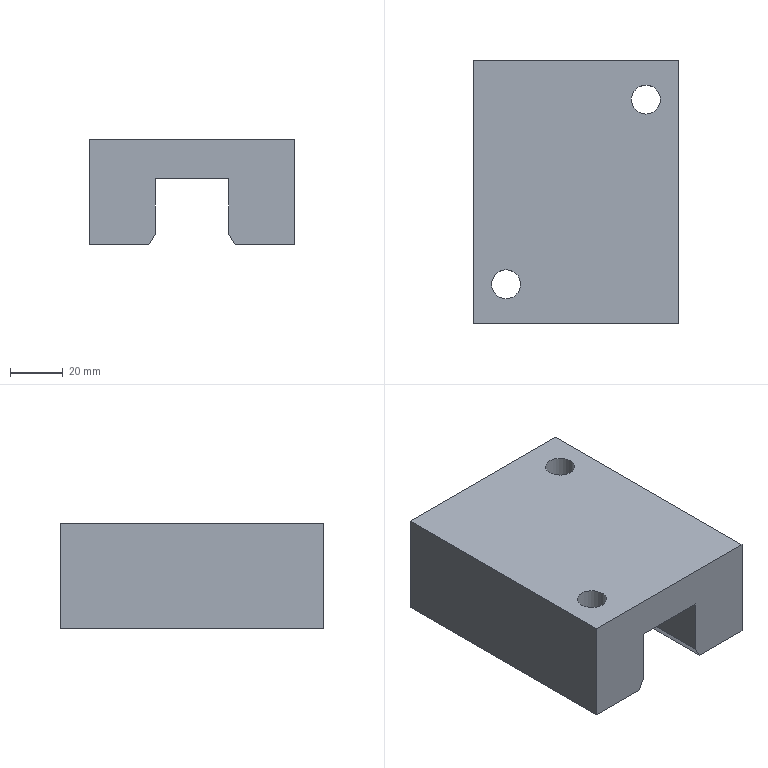Part | NX | features solid 2 | 1 solid | 18 faces | box 78 x 100 x 40 mm | volume 227096 mm3 | plane 14 | cylinder 4 | commonest cylinder face diameters 11 x2 18 x2
STEP:
#1=CARTESIAN_POINT('',(26.5,-551.,-690.));
#2=VERTEX_POINT('',#1);
#3=CARTESIAN_POINT('',(26.5,-560.,-690.));
#4=DIRECTION('',(0.,0.,-1.));
#5=DIRECTION('',(0.,1.,0.));
#6=AXIS2_PLACEMENT_3D('',#3,#4,#5);
#7=CIRCLE('',#6,9.);
#8=EDGE_CURVE('',#2,#2,#7,.F.);
#9=ORIENTED_EDGE('',*,*,#8,.T.);
#10=EDGE_LOOP('',(#9));
#11=FACE_BOUND('',#10,.T.);
#12=CARTESIAN_POINT('',(16.309,-645.,-690.));
#13=VERTEX_POINT('',#12);
#14=CARTESIAN_POINT('',(39.,-645.,-690.));
#15=VERTEX_POINT('',#14);
#16=CARTESIAN_POINT('',(-54.,-645.,-690.));
#17=DIRECTION('',(1.,0.,0.));
#18=VECTOR('',#17,1000.);
#19=LINE('',#16,#18);
#20=EDGE_CURVE('',#13,#15,#19,.T.);
#21=ORIENTED_EDGE('',*,*,#20,.F.);
#22=CARTESIAN_POINT('',(16.309,-545.,-690.));
#23=VERTEX_POINT('',#22);
#24=CARTESIAN_POINT('',(16.309,-961.874,-690.));
#25=DIRECTION('',(0.,1.,0.));
#26=VECTOR('',#25,1000.);
#27=LINE('',#24,#26);
#28=EDGE_CURVE('',#13,#23,#27,.T.);
#29=ORIENTED_EDGE('',*,*,#28,.T.);
#30=CARTESIAN_POINT('',(39.,-545.,-690.));
#31=VERTEX_POINT('',#30);
#32=CARTESIAN_POINT('',(-556.006,-545.,-690.));
#33=DIRECTION('',(-1.,0.,0.));
#34=VECTOR('',#33,1000.);
#35=LINE('',#32,#34);
#36=EDGE_CURVE('',#23,#31,#35,.F.);
#37=ORIENTED_EDGE('',*,*,#36,.T.);
#38=CARTESIAN_POINT('',(39.,-395.,-690.));
#39=DIRECTION('',(0.,-1.,0.));
#40=VECTOR('',#39,1000.);
#41=LINE('',#38,#40);
#42=EDGE_CURVE('',#31,#15,#41,.T.);
#43=ORIENTED_EDGE('',*,*,#42,.T.);
#44=EDGE_LOOP('',(#21,#29,#37,#43));
#45=FACE_BOUND('',#44,.T.);
#46=CARTESIAN_POINT('',(-556.006,-961.874,-690.));
#47=DIRECTION('',(0.,0.,-1.));
#48=DIRECTION('',(0.,1.,0.));
#49=AXIS2_PLACEMENT_3D('',#46,#47,#48);
#50=PLANE('',#49);
#51=ADVANCED_FACE('',(#11,#45),#50,.T.);
#52=CARTESIAN_POINT('',(-26.5,-639.,-690.));
#53=VERTEX_POINT('',#52);
#54=CARTESIAN_POINT('',(-26.5,-630.,-690.));
#55=DIRECTION('',(0.,0.,1.));
#56=DIRECTION('',(0.,-1.,0.));
#57=AXIS2_PLACEMENT_3D('',#54,#55,#56);
#58=CIRCLE('',#57,9.);
#59=EDGE_CURVE('',#53,#53,#58,.T.);
#60=ORIENTED_EDGE('',*,*,#59,.T.);
#61=EDGE_LOOP('',(#60));
#62=FACE_BOUND('',#61,.T.);
#63=CARTESIAN_POINT('',(-39.,-545.,-690.));
#64=VERTEX_POINT('',#63);
#65=CARTESIAN_POINT('',(-16.309,-545.,-690.));
#66=VERTEX_POINT('',#65);
#67=CARTESIAN_POINT('',(-556.006,-545.,-690.));
#68=DIRECTION('',(-1.,0.,0.));
#69=VECTOR('',#68,1000.);
#70=LINE('',#67,#69);
#71=EDGE_CURVE('',#64,#66,#70,.F.);
#72=ORIENTED_EDGE('',*,*,#71,.T.);
#73=CARTESIAN_POINT('',(-16.309,-645.,-690.));
#74=VERTEX_POINT('',#73);
#75=CARTESIAN_POINT('',(-16.309,-645.,-690.));
#76=DIRECTION('',(0.,-1.,0.));
#77=VECTOR('',#76,1000.);
#78=LINE('',#75,#77);
#79=EDGE_CURVE('',#66,#74,#78,.T.);
#80=ORIENTED_EDGE('',*,*,#79,.T.);
#81=CARTESIAN_POINT('',(-39.,-645.,-690.));
#82=VERTEX_POINT('',#81);
#83=CARTESIAN_POINT('',(-54.,-645.,-690.));
#84=DIRECTION('',(1.,0.,0.));
#85=VECTOR('',#84,1000.);
#86=LINE('',#83,#85);
#87=EDGE_CURVE('',#82,#74,#86,.T.);
#88=ORIENTED_EDGE('',*,*,#87,.F.);
#89=CARTESIAN_POINT('',(-39.,-395.,-690.));
#90=DIRECTION('',(0.,-1.,0.));
#91=VECTOR('',#90,1000.);
#92=LINE('',#89,#91);
#93=EDGE_CURVE('',#64,#82,#92,.T.);
#94=ORIENTED_EDGE('',*,*,#93,.F.);
#95=EDGE_LOOP('',(#72,#80,#88,#94));
#96=FACE_BOUND('',#95,.T.);
#97=CARTESIAN_POINT('',(-556.006,-961.874,-690.));
#98=DIRECTION('',(0.,0.,-1.));
#99=DIRECTION('',(0.,1.,0.));
#100=AXIS2_PLACEMENT_3D('',#97,#98,#99);
#101=PLANE('',#100);
#102=ADVANCED_FACE('',(#62,#96),#101,.T.);
#103=CARTESIAN_POINT('',(39.,-645.,-650.));
#104=VERTEX_POINT('',#103);
#105=CARTESIAN_POINT('',(39.,-545.,-650.));
#106=VERTEX_POINT('',#105);
#107=CARTESIAN_POINT('',(39.,-395.,-650.));
#108=DIRECTION('',(0.,1.,0.));
#109=VECTOR('',#108,1000.);
#110=LINE('',#107,#109);
#111=EDGE_CURVE('',#104,#106,#110,.T.);
#112=ORIENTED_EDGE('',*,*,#111,.F.);
#113=CARTESIAN_POINT('',(39.,-645.,-695.));
#114=DIRECTION('',(0.,0.,1.));
#115=VECTOR('',#114,1000.);
#116=LINE('',#113,#115);
#117=EDGE_CURVE('',#15,#104,#116,.T.);
#118=ORIENTED_EDGE('',*,*,#117,.F.);
#119=ORIENTED_EDGE('',*,*,#42,.F.);
#120=CARTESIAN_POINT('',(39.,-545.,-695.));
#121=DIRECTION('',(0.,0.,1.));
#122=VECTOR('',#121,1000.);
#123=LINE('',#120,#122);
#124=EDGE_CURVE('',#106,#31,#123,.F.);
#125=ORIENTED_EDGE('',*,*,#124,.F.);
#126=EDGE_LOOP('',(#112,#118,#119,#125));
#127=FACE_BOUND('',#126,.T.);
#128=CARTESIAN_POINT('',(39.,-395.,-695.));
#129=DIRECTION('',(-1.,0.,0.));
#130=DIRECTION('',(0.,0.,-1.));
#131=AXIS2_PLACEMENT_3D('',#128,#129,#130);
#132=PLANE('',#131);
#133=ADVANCED_FACE('',(#127),#132,.F.);
#134=CARTESIAN_POINT('',(-39.,-645.,-650.));
#135=VERTEX_POINT('',#134);
#136=CARTESIAN_POINT('',(-39.,-645.,-695.));
#137=DIRECTION('',(0.,0.,1.));
#138=VECTOR('',#137,1000.);
#139=LINE('',#136,#138);
#140=EDGE_CURVE('',#82,#135,#139,.T.);
#141=ORIENTED_EDGE('',*,*,#140,.T.);
#142=CARTESIAN_POINT('',(-39.,-545.,-650.));
#143=VERTEX_POINT('',#142);
#144=CARTESIAN_POINT('',(-39.,-440.,-650.));
#145=DIRECTION('',(0.,-1.,0.));
#146=VECTOR('',#145,1000.);
#147=LINE('',#144,#146);
#148=EDGE_CURVE('',#143,#135,#147,.T.);
#149=ORIENTED_EDGE('',*,*,#148,.F.);
#150=CARTESIAN_POINT('',(-39.,-545.,-690.));
#151=DIRECTION('',(0.,0.,-1.));
#152=VECTOR('',#151,1000.);
#153=LINE('',#150,#152);
#154=EDGE_CURVE('',#64,#143,#153,.F.);
#155=ORIENTED_EDGE('',*,*,#154,.F.);
#156=ORIENTED_EDGE('',*,*,#93,.T.);
#157=EDGE_LOOP('',(#141,#149,#155,#156));
#158=FACE_BOUND('',#157,.T.);
#159=CARTESIAN_POINT('',(-39.,-395.,-695.));
#160=DIRECTION('',(-1.,0.,0.));
#161=DIRECTION('',(0.,0.,-1.));
#162=AXIS2_PLACEMENT_3D('',#159,#160,#161);
#163=PLANE('',#162);
#164=ADVANCED_FACE('',(#158),#163,.T.);
#165=CARTESIAN_POINT('',(14.,-545.,-665.));
#166=VERTEX_POINT('',#165);
#167=CARTESIAN_POINT('',(-14.,-545.,-665.));
#168=VERTEX_POINT('',#167);
#169=CARTESIAN_POINT('',(0.,-545.,-665.));
#170=DIRECTION('',(-1.,0.,0.));
#171=VECTOR('',#170,1000.);
#172=LINE('',#169,#171);
#173=EDGE_CURVE('',#166,#168,#172,.T.);
#174=ORIENTED_EDGE('',*,*,#173,.F.);
#175=CARTESIAN_POINT('',(14.,-645.,-665.));
#176=VERTEX_POINT('',#175);
#177=CARTESIAN_POINT('',(14.,-395.,-665.));
#178=DIRECTION('',(0.,-1.,0.));
#179=VECTOR('',#178,1000.);
#180=LINE('',#177,#179);
#181=EDGE_CURVE('',#166,#176,#180,.T.);
#182=ORIENTED_EDGE('',*,*,#181,.T.);
#183=CARTESIAN_POINT('',(-14.,-645.,-665.));
#184=VERTEX_POINT('',#183);
#185=CARTESIAN_POINT('',(0.,-645.,-665.));
#186=DIRECTION('',(-1.,0.,0.));
#187=VECTOR('',#186,1000.);
#188=LINE('',#185,#187);
#189=EDGE_CURVE('',#184,#176,#188,.F.);
#190=ORIENTED_EDGE('',*,*,#189,.F.);
#191=CARTESIAN_POINT('',(-14.,-395.,-665.));
#192=DIRECTION('',(0.,-1.,0.));
#193=VECTOR('',#192,1000.);
#194=LINE('',#191,#193);
#195=EDGE_CURVE('',#168,#184,#194,.T.);
#196=ORIENTED_EDGE('',*,*,#195,.F.);
#197=EDGE_LOOP('',(#174,#182,#190,#196));
#198=FACE_BOUND('',#197,.T.);
#199=CARTESIAN_POINT('',(0.,-395.,-665.));
#200=DIRECTION('',(0.,0.,-1.));
#201=DIRECTION('',(0.,-1.,0.));
#202=AXIS2_PLACEMENT_3D('',#199,#200,#201);
#203=PLANE('',#202);
#204=ADVANCED_FACE('',(#198),#203,.T.);
#205=CARTESIAN_POINT('',(-14.,-645.,-686.));
#206=VERTEX_POINT('',#205);
#207=CARTESIAN_POINT('',(-14.,-645.,-695.));
#208=DIRECTION('',(0.,0.,1.));
#209=VECTOR('',#208,1000.);
#210=LINE('',#207,#209);
#211=EDGE_CURVE('',#206,#184,#210,.T.);
#212=ORIENTED_EDGE('',*,*,#211,.F.);
#213=CARTESIAN_POINT('',(-14.,-545.,-686.));
#214=VERTEX_POINT('',#213);
#215=CARTESIAN_POINT('',(-14.,-545.,-686.));
#216=DIRECTION('',(0.,1.,0.));
#217=VECTOR('',#216,1000.);
#218=LINE('',#215,#217);
#219=EDGE_CURVE('',#206,#214,#218,.T.);
#220=ORIENTED_EDGE('',*,*,#219,.T.);
#221=CARTESIAN_POINT('',(-14.,-545.,-690.));
#222=DIRECTION('',(0.,0.,1.));
#223=VECTOR('',#222,1000.);
#224=LINE('',#221,#223);
#225=EDGE_CURVE('',#168,#214,#224,.F.);
#226=ORIENTED_EDGE('',*,*,#225,.F.);
#227=ORIENTED_EDGE('',*,*,#195,.T.);
#228=EDGE_LOOP('',(#212,#220,#226,#227));
#229=FACE_BOUND('',#228,.T.);
#230=CARTESIAN_POINT('',(-14.,-395.,-690.));
#231=DIRECTION('',(-1.,0.,0.));
#232=DIRECTION('',(0.,0.,-1.));
#233=AXIS2_PLACEMENT_3D('',#230,#231,#232);
#234=PLANE('',#233);
#235=ADVANCED_FACE('',(#229),#234,.F.);
#236=CARTESIAN_POINT('',(14.,-545.,-686.));
#237=VERTEX_POINT('',#236);
#238=CARTESIAN_POINT('',(14.,-545.,-690.));
#239=DIRECTION('',(0.,0.,1.));
#240=VECTOR('',#239,1000.);
#241=LINE('',#238,#240);
#242=EDGE_CURVE('',#166,#237,#241,.F.);
#243=ORIENTED_EDGE('',*,*,#242,.T.);
#244=CARTESIAN_POINT('',(14.,-645.,-686.));
#245=VERTEX_POINT('',#244);
#246=CARTESIAN_POINT('',(14.,-395.,-686.));
#247=DIRECTION('',(0.,-1.,0.));
#248=VECTOR('',#247,1000.);
#249=LINE('',#246,#248);
#250=EDGE_CURVE('',#237,#245,#249,.T.);
#251=ORIENTED_EDGE('',*,*,#250,.T.);
#252=CARTESIAN_POINT('',(14.,-645.,-695.));
#253=DIRECTION('',(0.,0.,1.));
#254=VECTOR('',#253,1000.);
#255=LINE('',#252,#254);
#256=EDGE_CURVE('',#245,#176,#255,.T.);
#257=ORIENTED_EDGE('',*,*,#256,.T.);
#258=ORIENTED_EDGE('',*,*,#181,.F.);
#259=EDGE_LOOP('',(#243,#251,#257,#258));
#260=FACE_BOUND('',#259,.T.);
#261=CARTESIAN_POINT('',(14.,-395.,-690.));
#262=DIRECTION('',(-1.,0.,0.));
#263=DIRECTION('',(0.,0.,-1.));
#264=AXIS2_PLACEMENT_3D('',#261,#262,#263);
#265=PLANE('',#264);
#266=ADVANCED_FACE('',(#260),#265,.T.);
#267=CARTESIAN_POINT('',(-26.5,-635.5,-650.));
#268=VERTEX_POINT('',#267);
#269=CARTESIAN_POINT('',(-26.5,-630.,-650.));
#270=DIRECTION('',(0.,0.,1.));
#271=DIRECTION('',(0.,-1.,0.));
#272=AXIS2_PLACEMENT_3D('',#269,#270,#271);
#273=CIRCLE('',#272,5.5);
#274=EDGE_CURVE('',#268,#268,#273,.T.);
#275=ORIENTED_EDGE('',*,*,#274,.F.);
#276=EDGE_LOOP('',(#275));
#277=FACE_BOUND('',#276,.T.);
#278=CARTESIAN_POINT('',(26.5,-565.5,-650.));
#279=VERTEX_POINT('',#278);
#280=CARTESIAN_POINT('',(26.5,-560.,-650.));
#281=DIRECTION('',(0.,0.,1.));
#282=DIRECTION('',(0.,-1.,0.));
#283=AXIS2_PLACEMENT_3D('',#280,#281,#282);
#284=CIRCLE('',#283,5.5);
#285=EDGE_CURVE('',#279,#279,#284,.T.);
#286=ORIENTED_EDGE('',*,*,#285,.F.);
#287=EDGE_LOOP('',(#286));
#288=FACE_BOUND('',#287,.T.);
#289=CARTESIAN_POINT('',(-54.,-645.,-650.));
#290=DIRECTION('',(1.,0.,0.));
#291=VECTOR('',#290,1000.);
#292=LINE('',#289,#291);
#293=EDGE_CURVE('',#135,#104,#292,.T.);
#294=ORIENTED_EDGE('',*,*,#293,.T.);
#295=ORIENTED_EDGE('',*,*,#111,.T.);
#296=CARTESIAN_POINT('',(-54.,-545.,-650.));
#297=DIRECTION('',(-1.,0.,0.));
#298=VECTOR('',#297,1000.);
#299=LINE('',#296,#298);
#300=EDGE_CURVE('',#143,#106,#299,.F.);
#301=ORIENTED_EDGE('',*,*,#300,.F.);
#302=ORIENTED_EDGE('',*,*,#148,.T.);
#303=EDGE_LOOP('',(#294,#295,#301,#302));
#304=FACE_BOUND('',#303,.T.);
#305=CARTESIAN_POINT('',(-54.,-440.,-650.));
#306=DIRECTION('',(0.,0.,1.));
#307=DIRECTION('',(0.,-1.,0.));
#308=AXIS2_PLACEMENT_3D('',#305,#306,#307);
#309=PLANE('',#308);
#310=ADVANCED_FACE('',(#277,#288,#304),#309,.T.);
#311=ORIENTED_EDGE('',*,*,#256,.F.);
#312=CARTESIAN_POINT('',(-1.268,-645.,-659.555));
#313=DIRECTION('',(-0.5,0.,0.866));
#314=VECTOR('',#313,1000.);
#315=LINE('',#312,#314);
#316=EDGE_CURVE('',#245,#13,#315,.F.);
#317=ORIENTED_EDGE('',*,*,#316,.T.);
#318=ORIENTED_EDGE('',*,*,#20,.T.);
#319=ORIENTED_EDGE('',*,*,#117,.T.);
#320=ORIENTED_EDGE('',*,*,#293,.F.);
#321=ORIENTED_EDGE('',*,*,#140,.F.);
#322=ORIENTED_EDGE('',*,*,#87,.T.);
#323=CARTESIAN_POINT('',(-25.732,-645.,-706.321));
#324=DIRECTION('',(0.5,0.,0.866));
#325=VECTOR('',#324,1000.);
#326=LINE('',#323,#325);
#327=EDGE_CURVE('',#74,#206,#326,.T.);
#328=ORIENTED_EDGE('',*,*,#327,.T.);
#329=ORIENTED_EDGE('',*,*,#211,.T.);
#330=ORIENTED_EDGE('',*,*,#189,.T.);
#331=EDGE_LOOP('',(#311,#317,#318,#319,#320,#321,#322,#328,#329,#330));
#332=FACE_BOUND('',#331,.T.);
#333=CARTESIAN_POINT('',(-54.,-645.,-690.));
#334=DIRECTION('',(0.,-1.,0.));
#335=DIRECTION('',(1.,0.,0.));
#336=AXIS2_PLACEMENT_3D('',#333,#334,#335);
#337=PLANE('',#336);
#338=ADVANCED_FACE('',(#332),#337,.T.);
#339=ORIENTED_EDGE('',*,*,#36,.F.);
#340=CARTESIAN_POINT('',(-1.268,-545.,-659.555));
#341=DIRECTION('',(-0.5,0.,0.866));
#342=VECTOR('',#341,1000.);
#343=LINE('',#340,#342);
#344=EDGE_CURVE('',#23,#237,#343,.T.);
#345=ORIENTED_EDGE('',*,*,#344,.T.);
#346=ORIENTED_EDGE('',*,*,#242,.F.);
#347=ORIENTED_EDGE('',*,*,#173,.T.);
#348=ORIENTED_EDGE('',*,*,#225,.T.);
#349=CARTESIAN_POINT('',(-25.732,-545.,-706.321));
#350=DIRECTION('',(0.5,0.,0.866));
#351=VECTOR('',#350,1000.);
#352=LINE('',#349,#351);
#353=EDGE_CURVE('',#214,#66,#352,.F.);
#354=ORIENTED_EDGE('',*,*,#353,.T.);
#355=ORIENTED_EDGE('',*,*,#71,.F.);
#356=ORIENTED_EDGE('',*,*,#154,.T.);
#357=ORIENTED_EDGE('',*,*,#300,.T.);
#358=ORIENTED_EDGE('',*,*,#124,.T.);
#359=EDGE_LOOP('',(#339,#345,#346,#347,#348,#354,#355,#356,#357,#358));
#360=FACE_BOUND('',#359,.T.);
#361=CARTESIAN_POINT('',(-54.,-545.,-690.));
#362=DIRECTION('',(0.,-1.,0.));
#363=DIRECTION('',(1.,0.,0.));
#364=AXIS2_PLACEMENT_3D('',#361,#362,#363);
#365=PLANE('',#364);
#366=ADVANCED_FACE('',(#360),#365,.F.);
#367=ORIENTED_EDGE('',*,*,#285,.T.);
#368=EDGE_LOOP('',(#367));
#369=FACE_BOUND('',#368,.T.);
#370=CARTESIAN_POINT('',(26.5,-565.5,-670.));
#371=VERTEX_POINT('',#370);
#372=CARTESIAN_POINT('',(26.5,-560.,-670.));
#373=DIRECTION('',(0.,0.,1.));
#374=DIRECTION('',(0.,-1.,0.));
#375=AXIS2_PLACEMENT_3D('',#372,#373,#374);
#376=CIRCLE('',#375,5.5);
#377=EDGE_CURVE('',#371,#371,#376,.T.);
#378=ORIENTED_EDGE('',*,*,#377,.F.);
#379=EDGE_LOOP('',(#378));
#380=FACE_BOUND('',#379,.T.);
#381=CARTESIAN_POINT('',(26.5,-560.,-640.));
#382=DIRECTION('',(0.,0.,1.));
#383=DIRECTION('',(0.,-1.,0.));
#384=AXIS2_PLACEMENT_3D('',#381,#382,#383);
#385=CYLINDRICAL_SURFACE('',#384,5.5);
#386=ADVANCED_FACE('',(#369,#380),#385,.F.);
#387=ORIENTED_EDGE('',*,*,#377,.T.);
#388=EDGE_LOOP('',(#387));
#389=FACE_BOUND('',#388,.T.);
#390=CARTESIAN_POINT('',(26.5,-569.,-670.));
#391=VERTEX_POINT('',#390);
#392=CARTESIAN_POINT('',(26.5,-560.,-670.));
#393=DIRECTION('',(0.,0.,1.));
#394=DIRECTION('',(0.,-1.,0.));
#395=AXIS2_PLACEMENT_3D('',#392,#393,#394);
#396=CIRCLE('',#395,9.);
#397=EDGE_CURVE('',#391,#391,#396,.T.);
#398=ORIENTED_EDGE('',*,*,#397,.F.);
#399=EDGE_LOOP('',(#398));
#400=FACE_BOUND('',#399,.T.);
#401=CARTESIAN_POINT('',(24.,-560.,-670.));
#402=DIRECTION('',(0.,0.,1.));
#403=DIRECTION('',(0.,-1.,0.));
#404=AXIS2_PLACEMENT_3D('',#401,#402,#403);
#405=PLANE('',#404);
#406=ADVANCED_FACE('',(#389,#400),#405,.F.);
#407=ORIENTED_EDGE('',*,*,#397,.T.);
#408=EDGE_LOOP('',(#407));
#409=FACE_BOUND('',#408,.T.);
#410=ORIENTED_EDGE('',*,*,#8,.F.);
#411=EDGE_LOOP('',(#410));
#412=FACE_BOUND('',#411,.T.);
#413=CARTESIAN_POINT('',(26.5,-560.,-690.));
#414=DIRECTION('',(0.,0.,1.));
#415=DIRECTION('',(0.,-1.,0.));
#416=AXIS2_PLACEMENT_3D('',#413,#414,#415);
#417=CYLINDRICAL_SURFACE('',#416,9.);
#418=ADVANCED_FACE('',(#409,#412),#417,.F.);
#419=ORIENTED_EDGE('',*,*,#274,.T.);
#420=EDGE_LOOP('',(#419));
#421=FACE_BOUND('',#420,.T.);
#422=CARTESIAN_POINT('',(-26.5,-635.5,-670.));
#423=VERTEX_POINT('',#422);
#424=CARTESIAN_POINT('',(-26.5,-630.,-670.));
#425=DIRECTION('',(0.,0.,1.));
#426=DIRECTION('',(0.,-1.,0.));
#427=AXIS2_PLACEMENT_3D('',#424,#425,#426);
#428=CIRCLE('',#427,5.5);
#429=EDGE_CURVE('',#423,#423,#428,.T.);
#430=ORIENTED_EDGE('',*,*,#429,.F.);
#431=EDGE_LOOP('',(#430));
#432=FACE_BOUND('',#431,.T.);
#433=CARTESIAN_POINT('',(-26.5,-630.,-640.));
#434=DIRECTION('',(0.,0.,1.));
#435=DIRECTION('',(0.,-1.,0.));
#436=AXIS2_PLACEMENT_3D('',#433,#434,#435);
#437=CYLINDRICAL_SURFACE('',#436,5.5);
#438=ADVANCED_FACE('',(#421,#432),#437,.F.);
#439=ORIENTED_EDGE('',*,*,#429,.T.);
#440=EDGE_LOOP('',(#439));
#441=FACE_BOUND('',#440,.T.);
#442=CARTESIAN_POINT('',(-26.5,-639.,-670.));
#443=VERTEX_POINT('',#442);
#444=CARTESIAN_POINT('',(-26.5,-630.,-670.));
#445=DIRECTION('',(0.,0.,1.));
#446=DIRECTION('',(0.,-1.,0.));
#447=AXIS2_PLACEMENT_3D('',#444,#445,#446);
#448=CIRCLE('',#447,9.);
#449=EDGE_CURVE('',#443,#443,#448,.T.);
#450=ORIENTED_EDGE('',*,*,#449,.F.);
#451=EDGE_LOOP('',(#450));
#452=FACE_BOUND('',#451,.T.);
#453=CARTESIAN_POINT('',(-24.,-630.,-670.));
#454=DIRECTION('',(0.,0.,1.));
#455=DIRECTION('',(0.,-1.,0.));
#456=AXIS2_PLACEMENT_3D('',#453,#454,#455);
#457=PLANE('',#456);
#458=ADVANCED_FACE('',(#441,#452),#457,.F.);
#459=ORIENTED_EDGE('',*,*,#449,.T.);
#460=EDGE_LOOP('',(#459));
#461=FACE_BOUND('',#460,.T.);
#462=ORIENTED_EDGE('',*,*,#59,.F.);
#463=EDGE_LOOP('',(#462));
#464=FACE_BOUND('',#463,.T.);
#465=CARTESIAN_POINT('',(-26.5,-630.,-690.));
#466=DIRECTION('',(0.,0.,1.));
#467=DIRECTION('',(0.,-1.,0.));
#468=AXIS2_PLACEMENT_3D('',#465,#466,#467);
#469=CYLINDRICAL_SURFACE('',#468,9.);
#470=ADVANCED_FACE('',(#461,#464),#469,.F.);
#471=ORIENTED_EDGE('',*,*,#327,.F.);
#472=ORIENTED_EDGE('',*,*,#79,.F.);
#473=ORIENTED_EDGE('',*,*,#353,.F.);
#474=ORIENTED_EDGE('',*,*,#219,.F.);
#475=EDGE_LOOP('',(#471,#472,#473,#474));
#476=FACE_BOUND('',#475,.T.);
#477=CARTESIAN_POINT('',(-14.,-395.,-686.));
#478=DIRECTION('',(0.866,0.,-0.5));
#479=DIRECTION('',(0.5,0.,0.866));
#480=AXIS2_PLACEMENT_3D('',#477,#478,#479);
#481=PLANE('',#480);
#482=ADVANCED_FACE('',(#476),#481,.T.);
#483=ORIENTED_EDGE('',*,*,#316,.F.);
#484=ORIENTED_EDGE('',*,*,#250,.F.);
#485=ORIENTED_EDGE('',*,*,#344,.F.);
#486=ORIENTED_EDGE('',*,*,#28,.F.);
#487=EDGE_LOOP('',(#483,#484,#485,#486));
#488=FACE_BOUND('',#487,.T.);
#489=CARTESIAN_POINT('',(16.309,-961.874,-690.));
#490=DIRECTION('',(0.866,0.,0.5));
#491=DIRECTION('',(-0.5,0.,0.866));
#492=AXIS2_PLACEMENT_3D('',#489,#490,#491);
#493=PLANE('',#492);
#494=ADVANCED_FACE('',(#488),#493,.F.);
#495=CLOSED_SHELL('',(#51,#102,#133,#164,#204,#235,#266,#310,#338,#366,#386,#406,#418,#438,#458,#470,#482,#494));
#496=MANIFOLD_SOLID_BREP('',#495);
#497=(LENGTH_UNIT()NAMED_UNIT(*)SI_UNIT(.MILLI.,.METRE.));
#498=UNCERTAINTY_MEASURE_WITH_UNIT(LENGTH_MEASURE(0.00001),#497,'','');
#499=(NAMED_UNIT(*)PLANE_ANGLE_UNIT()SI_UNIT($,.RADIAN.));
#500=(NAMED_UNIT(*)SI_UNIT($,.STERADIAN.)SOLID_ANGLE_UNIT());
#501=(GEOMETRIC_REPRESENTATION_CONTEXT(3)GLOBAL_UNCERTAINTY_ASSIGNED_CONTEXT((#498))GLOBAL_UNIT_ASSIGNED_CONTEXT((#497,#499,#500))REPRESENTATION_CONTEXT('',''));
#502=ADVANCED_BREP_SHAPE_REPRESENTATION('',(#496),#501);